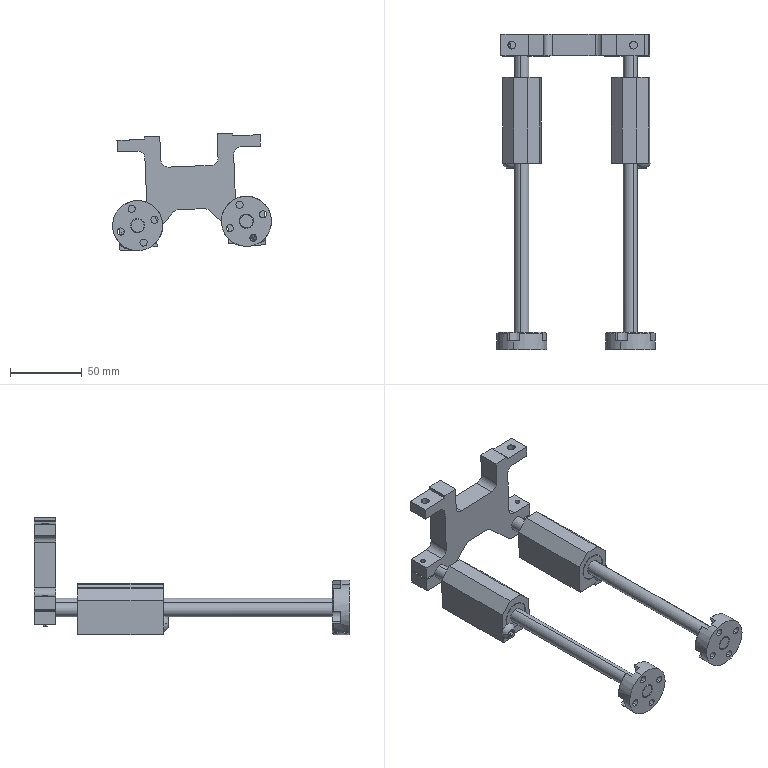Part | SolidWorks | 13 solids | 350 faces | box 110.938 x 220 x 82.039 mm | volume 184270 mm3 | plane 164 | cylinder 134 | cone 36 | spline 8 | sphere 4 | torus 4 | commonest cylinder face diameters 3.3 x28 10 x28 5 x16 19 x16 9 x10 18 x8